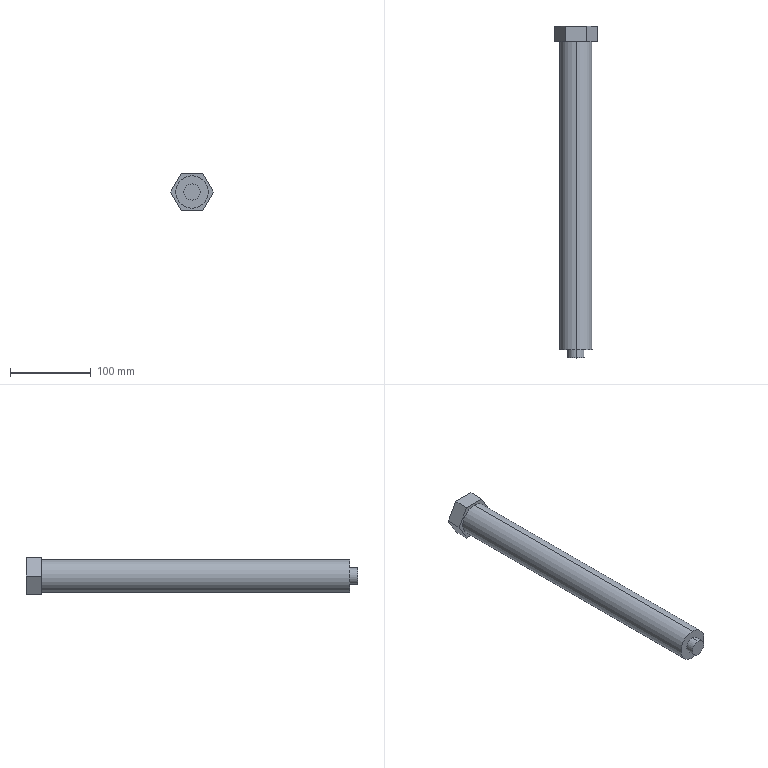Part | SolidWorks | features ICE 1, Revolution 1 | 1 solid | 14 faces | box 53 x 410 x 45.899 mm | volume 516586 mm3 | plane 10 | cylinder 4 | commonest cylinder face diameters 20 x2 40 x2
STEP:
#1=CARTESIAN_POINT('',(0.,391.,-20.));
#2=VERTEX_POINT('',#1);
#3=CARTESIAN_POINT('',(0.,391.,20.));
#4=VERTEX_POINT('',#3);
#5=CARTESIAN_POINT('',(0.,391.,0.));
#6=DIRECTION('',(0.,-1.,0.));
#7=DIRECTION('',(0.,0.,-1.));
#8=AXIS2_PLACEMENT_3D('',#5,#6,#7);
#9=CIRCLE('',#8,20.);
#10=EDGE_CURVE('',#2,#4,#9,.T.);
#11=ORIENTED_EDGE('',*,*,#10,.T.);
#12=CARTESIAN_POINT('',(0.,10.,20.));
#13=VERTEX_POINT('',#12);
#14=CARTESIAN_POINT('',(0.,0.,20.));
#15=DIRECTION('',(0.,-1.,0.));
#16=VECTOR('',#15,1000.);
#17=LINE('',#14,#16);
#18=EDGE_CURVE('',#4,#13,#17,.T.);
#19=ORIENTED_EDGE('',*,*,#18,.T.);
#20=CARTESIAN_POINT('',(0.,10.,-20.));
#21=VERTEX_POINT('',#20);
#22=CARTESIAN_POINT('',(0.,10.,0.));
#23=DIRECTION('',(0.,-1.,0.));
#24=DIRECTION('',(0.,0.,-1.));
#25=AXIS2_PLACEMENT_3D('',#22,#23,#24);
#26=CIRCLE('',#25,20.);
#27=EDGE_CURVE('',#21,#13,#26,.T.);
#28=ORIENTED_EDGE('',*,*,#27,.F.);
#29=CARTESIAN_POINT('',(0.,0.,-20.));
#30=DIRECTION('',(0.,-1.,0.));
#31=VECTOR('',#30,1000.);
#32=LINE('',#29,#31);
#33=EDGE_CURVE('',#2,#21,#32,.T.);
#34=ORIENTED_EDGE('',*,*,#33,.F.);
#35=EDGE_LOOP('',(#11,#19,#28,#34));
#36=FACE_OUTER_BOUND('',#35,.T.);
#37=CARTESIAN_POINT('',(0.,0.,0.));
#38=DIRECTION('',(0.,-1.,0.));
#39=DIRECTION('',(0.,0.,-1.));
#40=AXIS2_PLACEMENT_3D('',#37,#38,#39);
#41=CYLINDRICAL_SURFACE('',#40,20.);
#42=ADVANCED_FACE('',(#36),#41,.T.);
#43=CARTESIAN_POINT('',(0.,10.,-10.));
#44=VERTEX_POINT('',#43);
#45=CARTESIAN_POINT('',(0.,10.,10.));
#46=VERTEX_POINT('',#45);
#47=CARTESIAN_POINT('',(0.,10.,0.));
#48=DIRECTION('',(0.,-1.,0.));
#49=DIRECTION('',(0.,0.,-1.));
#50=AXIS2_PLACEMENT_3D('',#47,#48,#49);
#51=CIRCLE('',#50,10.);
#52=EDGE_CURVE('',#44,#46,#51,.T.);
#53=ORIENTED_EDGE('',*,*,#52,.T.);
#54=CARTESIAN_POINT('',(0.,0.,10.));
#55=VERTEX_POINT('',#54);
#56=CARTESIAN_POINT('',(0.,0.,10.));
#57=DIRECTION('',(0.,-1.,0.));
#58=VECTOR('',#57,1000.);
#59=LINE('',#56,#58);
#60=EDGE_CURVE('',#46,#55,#59,.T.);
#61=ORIENTED_EDGE('',*,*,#60,.T.);
#62=CARTESIAN_POINT('',(0.,0.,-10.));
#63=VERTEX_POINT('',#62);
#64=CARTESIAN_POINT('',(0.,0.,0.));
#65=DIRECTION('',(0.,-1.,0.));
#66=DIRECTION('',(0.,0.,-1.));
#67=AXIS2_PLACEMENT_3D('',#64,#65,#66);
#68=CIRCLE('',#67,10.);
#69=EDGE_CURVE('',#63,#55,#68,.T.);
#70=ORIENTED_EDGE('',*,*,#69,.F.);
#71=CARTESIAN_POINT('',(0.,0.,-10.));
#72=DIRECTION('',(0.,-1.,0.));
#73=VECTOR('',#72,1000.);
#74=LINE('',#71,#73);
#75=EDGE_CURVE('',#44,#63,#74,.T.);
#76=ORIENTED_EDGE('',*,*,#75,.F.);
#77=EDGE_LOOP('',(#53,#61,#70,#76));
#78=FACE_OUTER_BOUND('',#77,.T.);
#79=CARTESIAN_POINT('',(0.,0.,0.));
#80=DIRECTION('',(0.,-1.,0.));
#81=DIRECTION('',(0.,0.,-1.));
#82=AXIS2_PLACEMENT_3D('',#79,#80,#81);
#83=CYLINDRICAL_SURFACE('',#82,10.);
#84=ADVANCED_FACE('',(#78),#83,.T.);
#85=ORIENTED_EDGE('',*,*,#10,.F.);
#86=CARTESIAN_POINT('',(0.,391.,0.));
#87=DIRECTION('',(0.,-1.,0.));
#88=DIRECTION('',(0.,0.,-1.));
#89=AXIS2_PLACEMENT_3D('',#86,#87,#88);
#90=CIRCLE('',#89,20.);
#91=EDGE_CURVE('',#4,#2,#90,.T.);
#92=ORIENTED_EDGE('',*,*,#91,.F.);
#93=EDGE_LOOP('',(#85,#92));
#94=FACE_BOUND('',#93,.T.);
#95=CARTESIAN_POINT('',(-13.25,391.,22.95));
#96=VERTEX_POINT('',#95);
#97=CARTESIAN_POINT('',(-26.5,391.,0.));
#98=VERTEX_POINT('',#97);
#99=CARTESIAN_POINT('',(-14.875,391.,20.135));
#100=DIRECTION('',(-0.5,0.,-0.866));
#101=VECTOR('',#100,1000.);
#102=LINE('',#99,#101);
#103=EDGE_CURVE('',#96,#98,#102,.T.);
#104=ORIENTED_EDGE('',*,*,#103,.T.);
#105=CARTESIAN_POINT('',(-13.25,391.,-22.95));
#106=VERTEX_POINT('',#105);
#107=CARTESIAN_POINT('',(-14.875,391.,-20.135));
#108=DIRECTION('',(0.5,0.,-0.866));
#109=VECTOR('',#108,1000.);
#110=LINE('',#107,#109);
#111=EDGE_CURVE('',#98,#106,#110,.T.);
#112=ORIENTED_EDGE('',*,*,#111,.T.);
#113=CARTESIAN_POINT('',(13.25,391.,-22.95));
#114=VERTEX_POINT('',#113);
#115=CARTESIAN_POINT('',(20.,391.,-22.95));
#116=DIRECTION('',(1.,0.,0.));
#117=VECTOR('',#116,1000.);
#118=LINE('',#115,#117);
#119=EDGE_CURVE('',#106,#114,#118,.T.);
#120=ORIENTED_EDGE('',*,*,#119,.T.);
#121=CARTESIAN_POINT('',(26.5,391.,0.));
#122=VERTEX_POINT('',#121);
#123=CARTESIAN_POINT('',(24.875,391.,-2.815));
#124=DIRECTION('',(0.5,0.,0.866));
#125=VECTOR('',#124,1000.);
#126=LINE('',#123,#125);
#127=EDGE_CURVE('',#114,#122,#126,.T.);
#128=ORIENTED_EDGE('',*,*,#127,.T.);
#129=CARTESIAN_POINT('',(13.25,391.,22.95));
#130=VERTEX_POINT('',#129);
#131=CARTESIAN_POINT('',(24.875,391.,2.815));
#132=DIRECTION('',(-0.5,0.,0.866));
#133=VECTOR('',#132,1000.);
#134=LINE('',#131,#133);
#135=EDGE_CURVE('',#122,#130,#134,.T.);
#136=ORIENTED_EDGE('',*,*,#135,.T.);
#137=CARTESIAN_POINT('',(20.,391.,22.95));
#138=DIRECTION('',(-1.,0.,0.));
#139=VECTOR('',#138,1000.);
#140=LINE('',#137,#139);
#141=EDGE_CURVE('',#130,#96,#140,.T.);
#142=ORIENTED_EDGE('',*,*,#141,.T.);
#143=EDGE_LOOP('',(#104,#112,#120,#128,#136,#142));
#144=FACE_OUTER_BOUND('',#143,.T.);
#145=CARTESIAN_POINT('',(20.,391.,0.));
#146=DIRECTION('',(0.,-1.,0.));
#147=DIRECTION('',(0.,0.,-1.));
#148=AXIS2_PLACEMENT_3D('',#145,#146,#147);
#149=PLANE('',#148);
#150=ADVANCED_FACE('',(#94,#144),#149,.T.);
#151=ORIENTED_EDGE('',*,*,#69,.T.);
#152=CARTESIAN_POINT('',(0.,0.,0.));
#153=DIRECTION('',(0.,-1.,0.));
#154=DIRECTION('',(0.,0.,-1.));
#155=AXIS2_PLACEMENT_3D('',#152,#153,#154);
#156=CIRCLE('',#155,10.);
#157=EDGE_CURVE('',#55,#63,#156,.T.);
#158=ORIENTED_EDGE('',*,*,#157,.T.);
#159=EDGE_LOOP('',(#151,#158));
#160=FACE_OUTER_BOUND('',#159,.T.);
#161=CARTESIAN_POINT('',(0.,0.,0.));
#162=DIRECTION('',(0.,-1.,0.));
#163=DIRECTION('',(0.,0.,-1.));
#164=AXIS2_PLACEMENT_3D('',#161,#162,#163);
#165=PLANE('',#164);
#166=ADVANCED_FACE('',(#160),#165,.T.);
#167=ORIENTED_EDGE('',*,*,#60,.F.);
#168=CARTESIAN_POINT('',(0.,10.,0.));
#169=DIRECTION('',(0.,-1.,0.));
#170=DIRECTION('',(0.,0.,-1.));
#171=AXIS2_PLACEMENT_3D('',#168,#169,#170);
#172=CIRCLE('',#171,10.);
#173=EDGE_CURVE('',#46,#44,#172,.T.);
#174=ORIENTED_EDGE('',*,*,#173,.T.);
#175=ORIENTED_EDGE('',*,*,#75,.T.);
#176=ORIENTED_EDGE('',*,*,#157,.F.);
#177=EDGE_LOOP('',(#167,#174,#175,#176));
#178=FACE_OUTER_BOUND('',#177,.T.);
#179=CARTESIAN_POINT('',(0.,0.,0.));
#180=DIRECTION('',(0.,-1.,0.));
#181=DIRECTION('',(0.,0.,-1.));
#182=AXIS2_PLACEMENT_3D('',#179,#180,#181);
#183=CYLINDRICAL_SURFACE('',#182,10.);
#184=ADVANCED_FACE('',(#178),#183,.T.);
#185=ORIENTED_EDGE('',*,*,#27,.T.);
#186=CARTESIAN_POINT('',(0.,10.,0.));
#187=DIRECTION('',(0.,-1.,0.));
#188=DIRECTION('',(0.,0.,-1.));
#189=AXIS2_PLACEMENT_3D('',#186,#187,#188);
#190=CIRCLE('',#189,20.);
#191=EDGE_CURVE('',#13,#21,#190,.T.);
#192=ORIENTED_EDGE('',*,*,#191,.T.);
#193=EDGE_LOOP('',(#185,#192));
#194=FACE_OUTER_BOUND('',#193,.T.);
#195=ORIENTED_EDGE('',*,*,#52,.F.);
#196=ORIENTED_EDGE('',*,*,#173,.F.);
#197=EDGE_LOOP('',(#195,#196));
#198=FACE_BOUND('',#197,.T.);
#199=CARTESIAN_POINT('',(10.,10.,0.));
#200=DIRECTION('',(0.,-1.,0.));
#201=DIRECTION('',(0.,0.,-1.));
#202=AXIS2_PLACEMENT_3D('',#199,#200,#201);
#203=PLANE('',#202);
#204=ADVANCED_FACE('',(#194,#198),#203,.T.);
#205=ORIENTED_EDGE('',*,*,#18,.F.);
#206=ORIENTED_EDGE('',*,*,#91,.T.);
#207=ORIENTED_EDGE('',*,*,#33,.T.);
#208=ORIENTED_EDGE('',*,*,#191,.F.);
#209=EDGE_LOOP('',(#205,#206,#207,#208));
#210=FACE_OUTER_BOUND('',#209,.T.);
#211=CARTESIAN_POINT('',(0.,0.,0.));
#212=DIRECTION('',(0.,-1.,0.));
#213=DIRECTION('',(0.,0.,-1.));
#214=AXIS2_PLACEMENT_3D('',#211,#212,#213);
#215=CYLINDRICAL_SURFACE('',#214,20.);
#216=ADVANCED_FACE('',(#210),#215,.T.);
#217=CARTESIAN_POINT('',(-26.5,410.,0.));
#218=VERTEX_POINT('',#217);
#219=CARTESIAN_POINT('',(-26.5,378.,0.));
#220=DIRECTION('',(0.,1.,0.));
#221=VECTOR('',#220,1000.);
#222=LINE('',#219,#221);
#223=EDGE_CURVE('',#98,#218,#222,.T.);
#224=ORIENTED_EDGE('',*,*,#223,.T.);
#225=CARTESIAN_POINT('',(-13.25,410.,-22.95));
#226=VERTEX_POINT('',#225);
#227=CARTESIAN_POINT('',(-13.25,410.,-22.95));
#228=DIRECTION('',(-0.5,0.,0.866));
#229=VECTOR('',#228,1000.);
#230=LINE('',#227,#229);
#231=EDGE_CURVE('',#226,#218,#230,.T.);
#232=ORIENTED_EDGE('',*,*,#231,.F.);
#233=CARTESIAN_POINT('',(-13.25,378.,-22.95));
#234=DIRECTION('',(0.,1.,0.));
#235=VECTOR('',#234,1000.);
#236=LINE('',#233,#235);
#237=EDGE_CURVE('',#106,#226,#236,.T.);
#238=ORIENTED_EDGE('',*,*,#237,.F.);
#239=ORIENTED_EDGE('',*,*,#111,.F.);
#240=EDGE_LOOP('',(#224,#232,#238,#239));
#241=FACE_OUTER_BOUND('',#240,.T.);
#242=CARTESIAN_POINT('',(-13.25,378.,-22.95));
#243=DIRECTION('',(-0.866,0.,-0.5));
#244=DIRECTION('',(-0.5,0.,0.866));
#245=AXIS2_PLACEMENT_3D('',#242,#243,#244);
#246=PLANE('',#245);
#247=ADVANCED_FACE('',(#241),#246,.T.);
#248=ORIENTED_EDGE('',*,*,#237,.T.);
#249=CARTESIAN_POINT('',(13.25,410.,-22.95));
#250=VERTEX_POINT('',#249);
#251=CARTESIAN_POINT('',(13.25,410.,-22.95));
#252=DIRECTION('',(-1.,0.,0.));
#253=VECTOR('',#252,1000.);
#254=LINE('',#251,#253);
#255=EDGE_CURVE('',#250,#226,#254,.T.);
#256=ORIENTED_EDGE('',*,*,#255,.F.);
#257=CARTESIAN_POINT('',(13.25,378.,-22.95));
#258=DIRECTION('',(0.,1.,0.));
#259=VECTOR('',#258,1000.);
#260=LINE('',#257,#259);
#261=EDGE_CURVE('',#114,#250,#260,.T.);
#262=ORIENTED_EDGE('',*,*,#261,.F.);
#263=ORIENTED_EDGE('',*,*,#119,.F.);
#264=EDGE_LOOP('',(#248,#256,#262,#263));
#265=FACE_OUTER_BOUND('',#264,.T.);
#266=CARTESIAN_POINT('',(13.25,378.,-22.95));
#267=DIRECTION('',(0.,0.,-1.));
#268=DIRECTION('',(-1.,0.,0.));
#269=AXIS2_PLACEMENT_3D('',#266,#267,#268);
#270=PLANE('',#269);
#271=ADVANCED_FACE('',(#265),#270,.T.);
#272=ORIENTED_EDGE('',*,*,#261,.T.);
#273=CARTESIAN_POINT('',(26.5,410.,0.));
#274=VERTEX_POINT('',#273);
#275=CARTESIAN_POINT('',(26.5,410.,0.));
#276=DIRECTION('',(-0.5,0.,-0.866));
#277=VECTOR('',#276,1000.);
#278=LINE('',#275,#277);
#279=EDGE_CURVE('',#274,#250,#278,.T.);
#280=ORIENTED_EDGE('',*,*,#279,.F.);
#281=CARTESIAN_POINT('',(26.5,378.,0.));
#282=DIRECTION('',(0.,1.,0.));
#283=VECTOR('',#282,1000.);
#284=LINE('',#281,#283);
#285=EDGE_CURVE('',#122,#274,#284,.T.);
#286=ORIENTED_EDGE('',*,*,#285,.F.);
#287=ORIENTED_EDGE('',*,*,#127,.F.);
#288=EDGE_LOOP('',(#272,#280,#286,#287));
#289=FACE_OUTER_BOUND('',#288,.T.);
#290=CARTESIAN_POINT('',(26.5,378.,0.));
#291=DIRECTION('',(0.866,0.,-0.5));
#292=DIRECTION('',(-0.5,0.,-0.866));
#293=AXIS2_PLACEMENT_3D('',#290,#291,#292);
#294=PLANE('',#293);
#295=ADVANCED_FACE('',(#289),#294,.T.);
#296=ORIENTED_EDGE('',*,*,#285,.T.);
#297=CARTESIAN_POINT('',(13.25,410.,22.95));
#298=VERTEX_POINT('',#297);
#299=CARTESIAN_POINT('',(13.25,410.,22.95));
#300=DIRECTION('',(0.5,0.,-0.866));
#301=VECTOR('',#300,1000.);
#302=LINE('',#299,#301);
#303=EDGE_CURVE('',#298,#274,#302,.T.);
#304=ORIENTED_EDGE('',*,*,#303,.F.);
#305=CARTESIAN_POINT('',(13.25,378.,22.95));
#306=DIRECTION('',(0.,1.,0.));
#307=VECTOR('',#306,1000.);
#308=LINE('',#305,#307);
#309=EDGE_CURVE('',#130,#298,#308,.T.);
#310=ORIENTED_EDGE('',*,*,#309,.F.);
#311=ORIENTED_EDGE('',*,*,#135,.F.);
#312=EDGE_LOOP('',(#296,#304,#310,#311));
#313=FACE_OUTER_BOUND('',#312,.T.);
#314=CARTESIAN_POINT('',(13.25,378.,22.95));
#315=DIRECTION('',(0.866,0.,0.5));
#316=DIRECTION('',(0.5,0.,-0.866));
#317=AXIS2_PLACEMENT_3D('',#314,#315,#316);
#318=PLANE('',#317);
#319=ADVANCED_FACE('',(#313),#318,.T.);
#320=ORIENTED_EDGE('',*,*,#309,.T.);
#321=CARTESIAN_POINT('',(-13.25,410.,22.95));
#322=VERTEX_POINT('',#321);
#323=CARTESIAN_POINT('',(-13.25,410.,22.95));
#324=DIRECTION('',(1.,0.,0.));
#325=VECTOR('',#324,1000.);
#326=LINE('',#323,#325);
#327=EDGE_CURVE('',#322,#298,#326,.T.);
#328=ORIENTED_EDGE('',*,*,#327,.F.);
#329=CARTESIAN_POINT('',(-13.25,378.,22.95));
#330=DIRECTION('',(0.,1.,0.));
#331=VECTOR('',#330,1000.);
#332=LINE('',#329,#331);
#333=EDGE_CURVE('',#96,#322,#332,.T.);
#334=ORIENTED_EDGE('',*,*,#333,.F.);
#335=ORIENTED_EDGE('',*,*,#141,.F.);
#336=EDGE_LOOP('',(#320,#328,#334,#335));
#337=FACE_OUTER_BOUND('',#336,.T.);
#338=CARTESIAN_POINT('',(-13.25,378.,22.95));
#339=DIRECTION('',(0.,0.,1.));
#340=DIRECTION('',(1.,0.,0.));
#341=AXIS2_PLACEMENT_3D('',#338,#339,#340);
#342=PLANE('',#341);
#343=ADVANCED_FACE('',(#337),#342,.T.);
#344=ORIENTED_EDGE('',*,*,#333,.T.);
#345=CARTESIAN_POINT('',(-26.5,410.,0.));
#346=DIRECTION('',(0.5,0.,0.866));
#347=VECTOR('',#346,1000.);
#348=LINE('',#345,#347);
#349=EDGE_CURVE('',#218,#322,#348,.T.);
#350=ORIENTED_EDGE('',*,*,#349,.F.);
#351=ORIENTED_EDGE('',*,*,#223,.F.);
#352=ORIENTED_EDGE('',*,*,#103,.F.);
#353=EDGE_LOOP('',(#344,#350,#351,#352));
#354=FACE_OUTER_BOUND('',#353,.T.);
#355=CARTESIAN_POINT('',(-26.5,378.,0.));
#356=DIRECTION('',(-0.866,0.,0.5));
#357=DIRECTION('',(0.5,0.,0.866));
#358=AXIS2_PLACEMENT_3D('',#355,#356,#357);
#359=PLANE('',#358);
#360=ADVANCED_FACE('',(#354),#359,.T.);
#361=ORIENTED_EDGE('',*,*,#255,.T.);
#362=ORIENTED_EDGE('',*,*,#231,.T.);
#363=ORIENTED_EDGE('',*,*,#349,.T.);
#364=ORIENTED_EDGE('',*,*,#327,.T.);
#365=ORIENTED_EDGE('',*,*,#303,.T.);
#366=ORIENTED_EDGE('',*,*,#279,.T.);
#367=EDGE_LOOP('',(#361,#362,#363,#364,#365,#366));
#368=FACE_OUTER_BOUND('',#367,.T.);
#369=CARTESIAN_POINT('',(26.5,410.,0.));
#370=DIRECTION('',(0.,1.,0.));
#371=DIRECTION('',(0.,0.,1.));
#372=AXIS2_PLACEMENT_3D('',#369,#370,#371);
#373=PLANE('',#372);
#374=ADVANCED_FACE('',(#368),#373,.T.);
#375=CLOSED_SHELL('',(#42,#84,#150,#166,#184,#204,#216,#247,#271,#295,#319,#343,#360,#374));
#376=MANIFOLD_SOLID_BREP('',#375);
#377=CARTESIAN_POINT('',(0.,0.,0.));
#378=DIRECTION('',(0.,0.,1.));
#379=DIRECTION('',(1.,0.,0.));
#380=AXIS2_PLACEMENT_3D('',#377,#378,#379);
#381=(LENGTH_UNIT()NAMED_UNIT(*)SI_UNIT(.MILLI.,.METRE.));
#382=UNCERTAINTY_MEASURE_WITH_UNIT(LENGTH_MEASURE(0.00001),#381,'','');
#383=(NAMED_UNIT(*)PLANE_ANGLE_UNIT()SI_UNIT($,.RADIAN.));
#384=(NAMED_UNIT(*)SI_UNIT($,.STERADIAN.)SOLID_ANGLE_UNIT());
#385=(GEOMETRIC_REPRESENTATION_CONTEXT(3)GLOBAL_UNCERTAINTY_ASSIGNED_CONTEXT((#382))GLOBAL_UNIT_ASSIGNED_CONTEXT((#381,#383,#384))REPRESENTATION_CONTEXT('',''));
#386=ADVANCED_BREP_SHAPE_REPRESENTATION('',(#376,#380),#385);